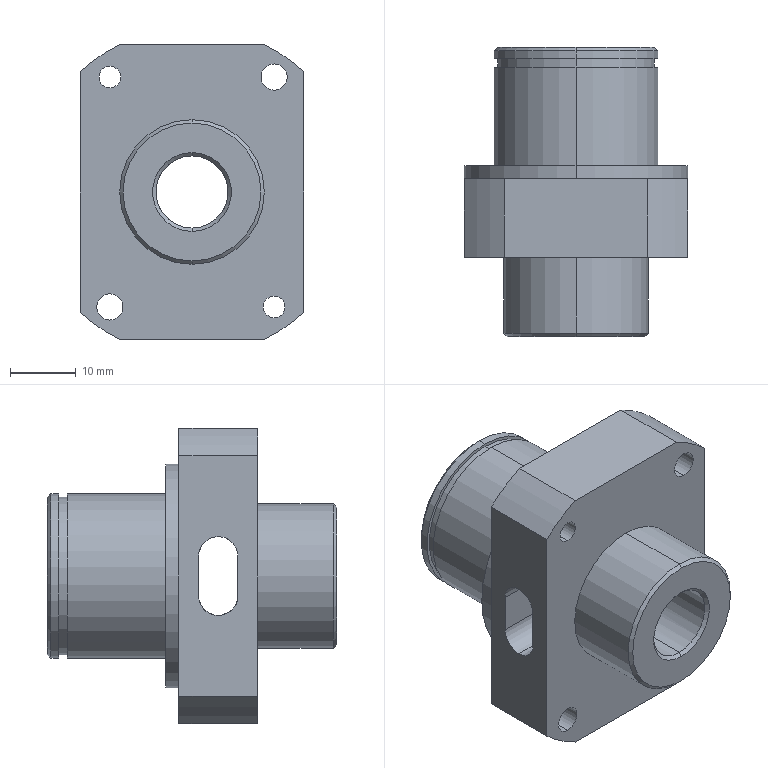Part | SolidWorks | features ICE 4, Chamfer 2, HoleWzd 1, Revolution 1 | 1 solid | 53 faces | box 34 x 44 x 45 mm | volume 26629 mm3 | cylinder 29 | plane 16 | cone 8 | commonest cylinder face diameters 3.3 x4 4 x4 11 x4 25 x4 50 x4 6 x3